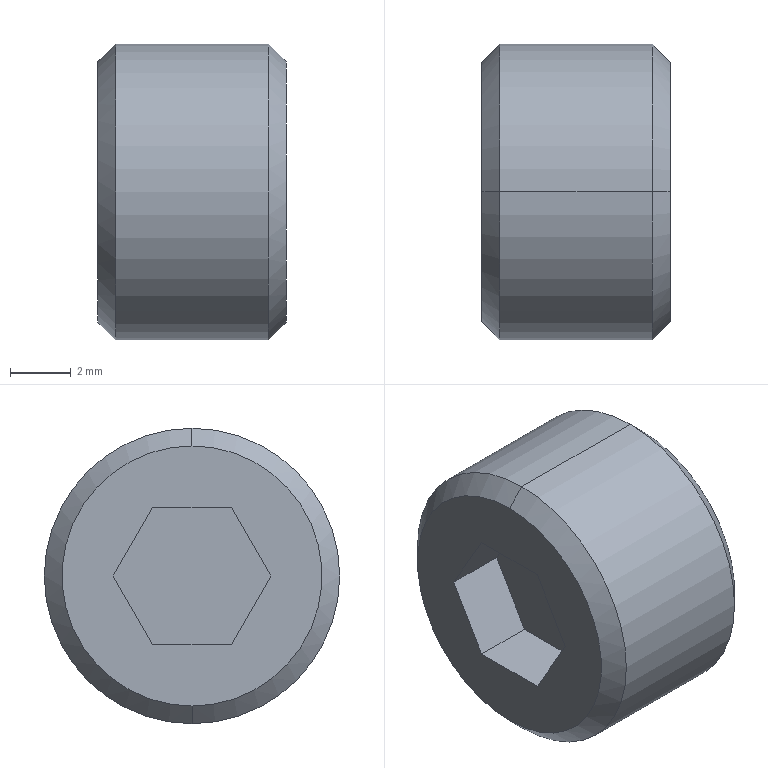Part | SolidWorks | features BaseBody 1 | 1 solid | 15 faces | box 6.2 x 9.728 x 9.728 mm | volume 415.838 mm3 | plane 9 | cone 4 | cylinder 2 | commonest cylinder face diameters 9.728 x2
STEP:
#1=CARTESIAN_POINT('',(5.619,0.,4.864));
#2=VERTEX_POINT('',#1);
#3=CARTESIAN_POINT('',(5.619,0.,-4.864));
#4=VERTEX_POINT('',#3);
#5=CARTESIAN_POINT('',(5.619,0.,0.));
#6=DIRECTION('',(-1.,0.,0.));
#7=DIRECTION('',(0.,0.,1.));
#8=AXIS2_PLACEMENT_3D('',#5,#6,#7);
#9=CIRCLE('',#8,4.864);
#10=EDGE_CURVE('',#2,#4,#9,.T.);
#11=ORIENTED_EDGE('',*,*,#10,.T.);
#12=CARTESIAN_POINT('',(0.581,0.,-4.864));
#13=VERTEX_POINT('',#12);
#14=CARTESIAN_POINT('',(6.2,0.,-4.864));
#15=DIRECTION('',(-1.,0.,0.));
#16=VECTOR('',#15,1000.);
#17=LINE('',#14,#16);
#18=EDGE_CURVE('',#4,#13,#17,.T.);
#19=ORIENTED_EDGE('',*,*,#18,.T.);
#20=CARTESIAN_POINT('',(0.581,0.,4.864));
#21=VERTEX_POINT('',#20);
#22=CARTESIAN_POINT('',(0.581,0.,0.));
#23=DIRECTION('',(1.,0.,0.));
#24=DIRECTION('',(0.,0.,1.));
#25=AXIS2_PLACEMENT_3D('',#22,#23,#24);
#26=CIRCLE('',#25,4.864);
#27=EDGE_CURVE('',#13,#21,#26,.T.);
#28=ORIENTED_EDGE('',*,*,#27,.T.);
#29=CARTESIAN_POINT('',(6.2,0.,4.864));
#30=DIRECTION('',(-1.,0.,0.));
#31=VECTOR('',#30,1000.);
#32=LINE('',#29,#31);
#33=EDGE_CURVE('',#2,#21,#32,.T.);
#34=ORIENTED_EDGE('',*,*,#33,.F.);
#35=EDGE_LOOP('',(#11,#19,#28,#34));
#36=FACE_OUTER_BOUND('',#35,.T.);
#37=CARTESIAN_POINT('',(6.2,0.,0.));
#38=DIRECTION('',(-1.,0.,0.));
#39=DIRECTION('',(0.,0.,1.));
#40=AXIS2_PLACEMENT_3D('',#37,#38,#39);
#41=CYLINDRICAL_SURFACE('',#40,4.864);
#42=ADVANCED_FACE('',(#36),#41,.T.);
#43=CARTESIAN_POINT('',(0.,0.,-4.283));
#44=VERTEX_POINT('',#43);
#45=CARTESIAN_POINT('',(0.,0.,4.283));
#46=VERTEX_POINT('',#45);
#47=CARTESIAN_POINT('',(0.,0.,0.));
#48=DIRECTION('',(1.,0.,0.));
#49=DIRECTION('',(0.,0.,-1.));
#50=AXIS2_PLACEMENT_3D('',#47,#48,#49);
#51=CIRCLE('',#50,4.283);
#52=EDGE_CURVE('',#44,#46,#51,.T.);
#53=ORIENTED_EDGE('',*,*,#52,.T.);
#54=CARTESIAN_POINT('',(0.581,0.,4.864));
#55=DIRECTION('',(0.7071,0.,0.7071));
#56=VECTOR('',#55,1000.);
#57=LINE('',#54,#56);
#58=EDGE_CURVE('',#46,#21,#57,.T.);
#59=ORIENTED_EDGE('',*,*,#58,.T.);
#60=ORIENTED_EDGE('',*,*,#27,.F.);
#61=CARTESIAN_POINT('',(0.581,0.,-4.864));
#62=DIRECTION('',(0.7071,0.,-0.7071));
#63=VECTOR('',#62,1000.);
#64=LINE('',#61,#63);
#65=EDGE_CURVE('',#44,#13,#64,.T.);
#66=ORIENTED_EDGE('',*,*,#65,.F.);
#67=EDGE_LOOP('',(#53,#59,#60,#66));
#68=FACE_OUTER_BOUND('',#67,.T.);
#69=CARTESIAN_POINT('',(0.581,0.,0.));
#70=DIRECTION('',(1.,0.,0.));
#71=DIRECTION('',(0.,0.,-1.));
#72=AXIS2_PLACEMENT_3D('',#69,#70,#71);
#73=CONICAL_SURFACE('',#72,4.864,0.7854);
#74=ADVANCED_FACE('',(#68),#73,.T.);
#75=CARTESIAN_POINT('',(6.2,0.,4.283));
#76=VERTEX_POINT('',#75);
#77=CARTESIAN_POINT('',(6.2,0.,-4.283));
#78=VERTEX_POINT('',#77);
#79=CARTESIAN_POINT('',(6.2,0.,0.));
#80=DIRECTION('',(-1.,0.,0.));
#81=DIRECTION('',(0.,0.,1.));
#82=AXIS2_PLACEMENT_3D('',#79,#80,#81);
#83=CIRCLE('',#82,4.283);
#84=EDGE_CURVE('',#76,#78,#83,.T.);
#85=ORIENTED_EDGE('',*,*,#84,.T.);
#86=CARTESIAN_POINT('',(5.619,0.,-4.864));
#87=DIRECTION('',(-0.7071,0.,-0.7071));
#88=VECTOR('',#87,1000.);
#89=LINE('',#86,#88);
#90=EDGE_CURVE('',#78,#4,#89,.T.);
#91=ORIENTED_EDGE('',*,*,#90,.T.);
#92=ORIENTED_EDGE('',*,*,#10,.F.);
#93=CARTESIAN_POINT('',(5.619,0.,4.864));
#94=DIRECTION('',(-0.7071,0.,0.7071));
#95=VECTOR('',#94,1000.);
#96=LINE('',#93,#95);
#97=EDGE_CURVE('',#76,#2,#96,.T.);
#98=ORIENTED_EDGE('',*,*,#97,.F.);
#99=EDGE_LOOP('',(#85,#91,#92,#98));
#100=FACE_OUTER_BOUND('',#99,.T.);
#101=CARTESIAN_POINT('',(5.619,0.,0.));
#102=DIRECTION('',(-1.,0.,0.));
#103=DIRECTION('',(0.,0.,1.));
#104=AXIS2_PLACEMENT_3D('',#101,#102,#103);
#105=CONICAL_SURFACE('',#104,4.864,0.7854);
#106=ADVANCED_FACE('',(#100),#105,.T.);
#107=ORIENTED_EDGE('',*,*,#18,.F.);
#108=CARTESIAN_POINT('',(5.619,0.,0.));
#109=DIRECTION('',(-1.,0.,0.));
#110=DIRECTION('',(0.,0.,1.));
#111=AXIS2_PLACEMENT_3D('',#108,#109,#110);
#112=CIRCLE('',#111,4.864);
#113=EDGE_CURVE('',#4,#2,#112,.T.);
#114=ORIENTED_EDGE('',*,*,#113,.T.);
#115=ORIENTED_EDGE('',*,*,#33,.T.);
#116=CARTESIAN_POINT('',(0.581,0.,0.));
#117=DIRECTION('',(1.,0.,0.));
#118=DIRECTION('',(0.,0.,1.));
#119=AXIS2_PLACEMENT_3D('',#116,#117,#118);
#120=CIRCLE('',#119,4.864);
#121=EDGE_CURVE('',#21,#13,#120,.T.);
#122=ORIENTED_EDGE('',*,*,#121,.T.);
#123=EDGE_LOOP('',(#107,#114,#115,#122));
#124=FACE_OUTER_BOUND('',#123,.T.);
#125=CARTESIAN_POINT('',(6.2,0.,0.));
#126=DIRECTION('',(-1.,0.,0.));
#127=DIRECTION('',(0.,0.,1.));
#128=AXIS2_PLACEMENT_3D('',#125,#126,#127);
#129=CYLINDRICAL_SURFACE('',#128,4.864);
#130=ADVANCED_FACE('',(#124),#129,.T.);
#131=ORIENTED_EDGE('',*,*,#58,.F.);
#132=CARTESIAN_POINT('',(0.,0.,0.));
#133=DIRECTION('',(1.,0.,0.));
#134=DIRECTION('',(0.,0.,-1.));
#135=AXIS2_PLACEMENT_3D('',#132,#133,#134);
#136=CIRCLE('',#135,4.283);
#137=EDGE_CURVE('',#46,#44,#136,.T.);
#138=ORIENTED_EDGE('',*,*,#137,.T.);
#139=ORIENTED_EDGE('',*,*,#65,.T.);
#140=ORIENTED_EDGE('',*,*,#121,.F.);
#141=EDGE_LOOP('',(#131,#138,#139,#140));
#142=FACE_OUTER_BOUND('',#141,.T.);
#143=CARTESIAN_POINT('',(0.581,0.,0.));
#144=DIRECTION('',(1.,0.,0.));
#145=DIRECTION('',(0.,0.,-1.));
#146=AXIS2_PLACEMENT_3D('',#143,#144,#145);
#147=CONICAL_SURFACE('',#146,4.864,0.7854);
#148=ADVANCED_FACE('',(#142),#147,.T.);
#149=ORIENTED_EDGE('',*,*,#90,.F.);
#150=CARTESIAN_POINT('',(6.2,0.,0.));
#151=DIRECTION('',(-1.,0.,0.));
#152=DIRECTION('',(0.,0.,1.));
#153=AXIS2_PLACEMENT_3D('',#150,#151,#152);
#154=CIRCLE('',#153,4.283);
#155=EDGE_CURVE('',#78,#76,#154,.T.);
#156=ORIENTED_EDGE('',*,*,#155,.T.);
#157=ORIENTED_EDGE('',*,*,#97,.T.);
#158=ORIENTED_EDGE('',*,*,#113,.F.);
#159=EDGE_LOOP('',(#149,#156,#157,#158));
#160=FACE_OUTER_BOUND('',#159,.T.);
#161=CARTESIAN_POINT('',(5.619,0.,0.));
#162=DIRECTION('',(-1.,0.,0.));
#163=DIRECTION('',(0.,0.,1.));
#164=AXIS2_PLACEMENT_3D('',#161,#162,#163);
#165=CONICAL_SURFACE('',#164,4.864,0.7854);
#166=ADVANCED_FACE('',(#160),#165,.T.);
#167=CARTESIAN_POINT('',(0.,-2.598,0.));
#168=VERTEX_POINT('',#167);
#169=CARTESIAN_POINT('',(0.,-1.299,2.25));
#170=VERTEX_POINT('',#169);
#171=CARTESIAN_POINT('',(0.,-2.598,0.));
#172=DIRECTION('',(0.,0.5,0.866));
#173=VECTOR('',#172,1000.);
#174=LINE('',#171,#173);
#175=EDGE_CURVE('',#168,#170,#174,.T.);
#176=ORIENTED_EDGE('',*,*,#175,.F.);
#177=CARTESIAN_POINT('',(0.,-1.299,-2.25));
#178=VERTEX_POINT('',#177);
#179=CARTESIAN_POINT('',(0.,-1.299,-2.25));
#180=DIRECTION('',(0.,-0.5,0.866));
#181=VECTOR('',#180,1000.);
#182=LINE('',#179,#181);
#183=EDGE_CURVE('',#178,#168,#182,.T.);
#184=ORIENTED_EDGE('',*,*,#183,.F.);
#185=CARTESIAN_POINT('',(0.,1.299,-2.25));
#186=VERTEX_POINT('',#185);
#187=CARTESIAN_POINT('',(0.,0.,-2.25));
#188=DIRECTION('',(0.,-1.,0.));
#189=VECTOR('',#188,1000.);
#190=LINE('',#187,#189);
#191=EDGE_CURVE('',#186,#178,#190,.T.);
#192=ORIENTED_EDGE('',*,*,#191,.F.);
#193=CARTESIAN_POINT('',(0.,2.598,0.));
#194=VERTEX_POINT('',#193);
#195=CARTESIAN_POINT('',(0.,2.598,0.));
#196=DIRECTION('',(0.,-0.5,-0.866));
#197=VECTOR('',#196,1000.);
#198=LINE('',#195,#197);
#199=EDGE_CURVE('',#194,#186,#198,.T.);
#200=ORIENTED_EDGE('',*,*,#199,.F.);
#201=CARTESIAN_POINT('',(0.,1.299,2.25));
#202=VERTEX_POINT('',#201);
#203=CARTESIAN_POINT('',(0.,1.299,2.25));
#204=DIRECTION('',(0.,0.5,-0.866));
#205=VECTOR('',#204,1000.);
#206=LINE('',#203,#205);
#207=EDGE_CURVE('',#202,#194,#206,.T.);
#208=ORIENTED_EDGE('',*,*,#207,.F.);
#209=CARTESIAN_POINT('',(0.,0.,2.25));
#210=DIRECTION('',(0.,1.,0.));
#211=VECTOR('',#210,1000.);
#212=LINE('',#209,#211);
#213=EDGE_CURVE('',#170,#202,#212,.T.);
#214=ORIENTED_EDGE('',*,*,#213,.F.);
#215=EDGE_LOOP('',(#176,#184,#192,#200,#208,#214));
#216=FACE_BOUND('',#215,.T.);
#217=ORIENTED_EDGE('',*,*,#52,.F.);
#218=ORIENTED_EDGE('',*,*,#137,.F.);
#219=EDGE_LOOP('',(#217,#218));
#220=FACE_OUTER_BOUND('',#219,.T.);
#221=CARTESIAN_POINT('',(0.,0.,0.));
#222=DIRECTION('',(1.,0.,0.));
#223=DIRECTION('',(0.,0.,-1.));
#224=AXIS2_PLACEMENT_3D('',#221,#222,#223);
#225=PLANE('',#224);
#226=ADVANCED_FACE('',(#216,#220),#225,.F.);
#227=ORIENTED_EDGE('',*,*,#84,.F.);
#228=ORIENTED_EDGE('',*,*,#155,.F.);
#229=EDGE_LOOP('',(#227,#228));
#230=FACE_OUTER_BOUND('',#229,.T.);
#231=CARTESIAN_POINT('',(6.2,4.283,0.));
#232=DIRECTION('',(-1.,0.,0.));
#233=DIRECTION('',(0.,0.,1.));
#234=AXIS2_PLACEMENT_3D('',#231,#232,#233);
#235=PLANE('',#234);
#236=ADVANCED_FACE('',(#230),#235,.F.);
#237=CARTESIAN_POINT('',(2.,1.299,2.25));
#238=VERTEX_POINT('',#237);
#239=CARTESIAN_POINT('',(2.,-1.299,2.25));
#240=VERTEX_POINT('',#239);
#241=CARTESIAN_POINT('',(2.,1.299,2.25));
#242=DIRECTION('',(0.,-1.,0.));
#243=VECTOR('',#242,1000.);
#244=LINE('',#241,#243);
#245=EDGE_CURVE('',#238,#240,#244,.T.);
#246=ORIENTED_EDGE('',*,*,#245,.T.);
#247=CARTESIAN_POINT('',(2.,-1.299,2.25));
#248=DIRECTION('',(-1.,0.,0.));
#249=VECTOR('',#248,1000.);
#250=LINE('',#247,#249);
#251=EDGE_CURVE('',#240,#170,#250,.T.);
#252=ORIENTED_EDGE('',*,*,#251,.T.);
#253=ORIENTED_EDGE('',*,*,#213,.T.);
#254=CARTESIAN_POINT('',(2.,1.299,2.25));
#255=DIRECTION('',(1.,0.,0.));
#256=VECTOR('',#255,1000.);
#257=LINE('',#254,#256);
#258=EDGE_CURVE('',#202,#238,#257,.T.);
#259=ORIENTED_EDGE('',*,*,#258,.T.);
#260=EDGE_LOOP('',(#246,#252,#253,#259));
#261=FACE_OUTER_BOUND('',#260,.T.);
#262=CARTESIAN_POINT('',(2.,1.299,2.25));
#263=DIRECTION('',(0.,0.,-1.));
#264=DIRECTION('',(-1.,0.,0.));
#265=AXIS2_PLACEMENT_3D('',#262,#263,#264);
#266=PLANE('',#265);
#267=ADVANCED_FACE('',(#261),#266,.T.);
#268=CARTESIAN_POINT('',(2.,-2.598,0.));
#269=VERTEX_POINT('',#268);
#270=CARTESIAN_POINT('',(2.,-1.299,2.25));
#271=DIRECTION('',(0.,-0.5,-0.866));
#272=VECTOR('',#271,1000.);
#273=LINE('',#270,#272);
#274=EDGE_CURVE('',#240,#269,#273,.T.);
#275=ORIENTED_EDGE('',*,*,#274,.T.);
#276=CARTESIAN_POINT('',(2.,-2.598,0.));
#277=DIRECTION('',(-1.,0.,0.));
#278=VECTOR('',#277,1000.);
#279=LINE('',#276,#278);
#280=EDGE_CURVE('',#269,#168,#279,.T.);
#281=ORIENTED_EDGE('',*,*,#280,.T.);
#282=ORIENTED_EDGE('',*,*,#175,.T.);
#283=ORIENTED_EDGE('',*,*,#251,.F.);
#284=EDGE_LOOP('',(#275,#281,#282,#283));
#285=FACE_OUTER_BOUND('',#284,.T.);
#286=CARTESIAN_POINT('',(2.,-1.299,2.25));
#287=DIRECTION('',(0.,0.866,-0.5));
#288=DIRECTION('',(0.,0.5,0.866));
#289=AXIS2_PLACEMENT_3D('',#286,#287,#288);
#290=PLANE('',#289);
#291=ADVANCED_FACE('',(#285),#290,.T.);
#292=CARTESIAN_POINT('',(2.,-1.299,-2.25));
#293=VERTEX_POINT('',#292);
#294=CARTESIAN_POINT('',(2.,-2.598,0.));
#295=DIRECTION('',(0.,0.5,-0.866));
#296=VECTOR('',#295,1000.);
#297=LINE('',#294,#296);
#298=EDGE_CURVE('',#269,#293,#297,.T.);
#299=ORIENTED_EDGE('',*,*,#298,.T.);
#300=CARTESIAN_POINT('',(2.,-1.299,-2.25));
#301=DIRECTION('',(-1.,0.,0.));
#302=VECTOR('',#301,1000.);
#303=LINE('',#300,#302);
#304=EDGE_CURVE('',#293,#178,#303,.T.);
#305=ORIENTED_EDGE('',*,*,#304,.T.);
#306=ORIENTED_EDGE('',*,*,#183,.T.);
#307=ORIENTED_EDGE('',*,*,#280,.F.);
#308=EDGE_LOOP('',(#299,#305,#306,#307));
#309=FACE_OUTER_BOUND('',#308,.T.);
#310=CARTESIAN_POINT('',(2.,-2.598,0.));
#311=DIRECTION('',(0.,0.866,0.5));
#312=DIRECTION('',(0.,-0.5,0.866));
#313=AXIS2_PLACEMENT_3D('',#310,#311,#312);
#314=PLANE('',#313);
#315=ADVANCED_FACE('',(#309),#314,.T.);
#316=CARTESIAN_POINT('',(2.,1.299,-2.25));
#317=VERTEX_POINT('',#316);
#318=CARTESIAN_POINT('',(2.,-1.299,-2.25));
#319=DIRECTION('',(0.,1.,0.));
#320=VECTOR('',#319,1000.);
#321=LINE('',#318,#320);
#322=EDGE_CURVE('',#293,#317,#321,.T.);
#323=ORIENTED_EDGE('',*,*,#322,.T.);
#324=CARTESIAN_POINT('',(2.,1.299,-2.25));
#325=DIRECTION('',(-1.,0.,0.));
#326=VECTOR('',#325,1000.);
#327=LINE('',#324,#326);
#328=EDGE_CURVE('',#317,#186,#327,.T.);
#329=ORIENTED_EDGE('',*,*,#328,.T.);
#330=ORIENTED_EDGE('',*,*,#191,.T.);
#331=ORIENTED_EDGE('',*,*,#304,.F.);
#332=EDGE_LOOP('',(#323,#329,#330,#331));
#333=FACE_OUTER_BOUND('',#332,.T.);
#334=CARTESIAN_POINT('',(2.,-1.299,-2.25));
#335=DIRECTION('',(0.,0.,1.));
#336=DIRECTION('',(1.,0.,0.));
#337=AXIS2_PLACEMENT_3D('',#334,#335,#336);
#338=PLANE('',#337);
#339=ADVANCED_FACE('',(#333),#338,.T.);
#340=CARTESIAN_POINT('',(2.,2.598,0.));
#341=VERTEX_POINT('',#340);
#342=CARTESIAN_POINT('',(2.,1.299,-2.25));
#343=DIRECTION('',(0.,0.5,0.866));
#344=VECTOR('',#343,1000.);
#345=LINE('',#342,#344);
#346=EDGE_CURVE('',#317,#341,#345,.T.);
#347=ORIENTED_EDGE('',*,*,#346,.T.);
#348=CARTESIAN_POINT('',(2.,2.598,0.));
#349=DIRECTION('',(-1.,0.,0.));
#350=VECTOR('',#349,1000.);
#351=LINE('',#348,#350);
#352=EDGE_CURVE('',#341,#194,#351,.T.);
#353=ORIENTED_EDGE('',*,*,#352,.T.);
#354=ORIENTED_EDGE('',*,*,#199,.T.);
#355=ORIENTED_EDGE('',*,*,#328,.F.);
#356=EDGE_LOOP('',(#347,#353,#354,#355));
#357=FACE_OUTER_BOUND('',#356,.T.);
#358=CARTESIAN_POINT('',(2.,1.299,-2.25));
#359=DIRECTION('',(0.,-0.866,0.5));
#360=DIRECTION('',(0.,-0.5,-0.866));
#361=AXIS2_PLACEMENT_3D('',#358,#359,#360);
#362=PLANE('',#361);
#363=ADVANCED_FACE('',(#357),#362,.T.);
#364=CARTESIAN_POINT('',(2.,2.598,0.));
#365=DIRECTION('',(0.,-0.5,0.866));
#366=VECTOR('',#365,1000.);
#367=LINE('',#364,#366);
#368=EDGE_CURVE('',#341,#238,#367,.T.);
#369=ORIENTED_EDGE('',*,*,#368,.T.);
#370=ORIENTED_EDGE('',*,*,#258,.F.);
#371=ORIENTED_EDGE('',*,*,#207,.T.);
#372=ORIENTED_EDGE('',*,*,#352,.F.);
#373=EDGE_LOOP('',(#369,#370,#371,#372));
#374=FACE_OUTER_BOUND('',#373,.T.);
#375=CARTESIAN_POINT('',(2.,2.598,0.));
#376=DIRECTION('',(0.,-0.866,-0.5));
#377=DIRECTION('',(0.,0.5,-0.866));
#378=AXIS2_PLACEMENT_3D('',#375,#376,#377);
#379=PLANE('',#378);
#380=ADVANCED_FACE('',(#374),#379,.T.);
#381=ORIENTED_EDGE('',*,*,#368,.F.);
#382=ORIENTED_EDGE('',*,*,#346,.F.);
#383=ORIENTED_EDGE('',*,*,#322,.F.);
#384=ORIENTED_EDGE('',*,*,#298,.F.);
#385=ORIENTED_EDGE('',*,*,#274,.F.);
#386=ORIENTED_EDGE('',*,*,#245,.F.);
#387=EDGE_LOOP('',(#381,#382,#383,#384,#385,#386));
#388=FACE_OUTER_BOUND('',#387,.T.);
#389=CARTESIAN_POINT('',(2.,0.,0.));
#390=DIRECTION('',(1.,0.,0.));
#391=DIRECTION('',(0.,0.,-1.));
#392=AXIS2_PLACEMENT_3D('',#389,#390,#391);
#393=PLANE('',#392);
#394=ADVANCED_FACE('',(#388),#393,.F.);
#395=CLOSED_SHELL('',(#42,#74,#106,#130,#148,#166,#226,#236,#267,#291,#315,#339,#363,#380,#394));
#396=MANIFOLD_SOLID_BREP('',#395);
#397=CARTESIAN_POINT('',(0.,0.,0.));
#398=DIRECTION('',(0.,0.,1.));
#399=DIRECTION('',(1.,0.,0.));
#400=AXIS2_PLACEMENT_3D('',#397,#398,#399);
#401=(LENGTH_UNIT()NAMED_UNIT(*)SI_UNIT(.MILLI.,.METRE.));
#402=UNCERTAINTY_MEASURE_WITH_UNIT(LENGTH_MEASURE(0.00001),#401,'','');
#403=(NAMED_UNIT(*)PLANE_ANGLE_UNIT()SI_UNIT($,.RADIAN.));
#404=(NAMED_UNIT(*)SI_UNIT($,.STERADIAN.)SOLID_ANGLE_UNIT());
#405=(GEOMETRIC_REPRESENTATION_CONTEXT(3)GLOBAL_UNCERTAINTY_ASSIGNED_CONTEXT((#402))GLOBAL_UNIT_ASSIGNED_CONTEXT((#401,#403,#404))REPRESENTATION_CONTEXT('',''));
#406=ADVANCED_BREP_SHAPE_REPRESENTATION('',(#396,#400),#405);